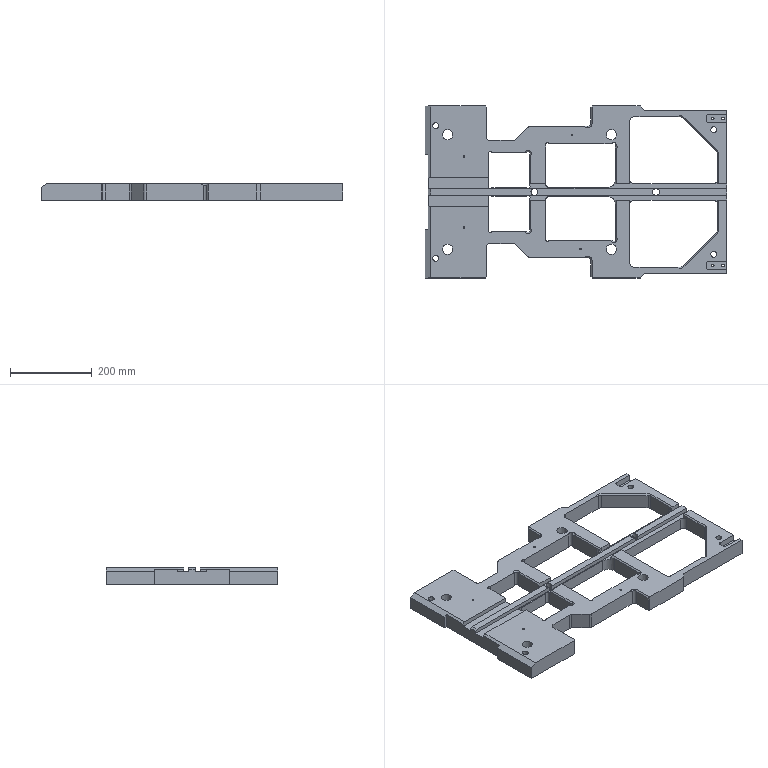Part | STEP file | lll_id4578_x_t | 1 solid | 217 faces | box 737.308 x 420 x 40 mm | volume 5836946 mm3 | plane 120 | cylinder 75 | cone 22 | commonest cylinder face diameters 10 x16 16 x11 20 x10 6.806 x4 14 x4 14.506 x4